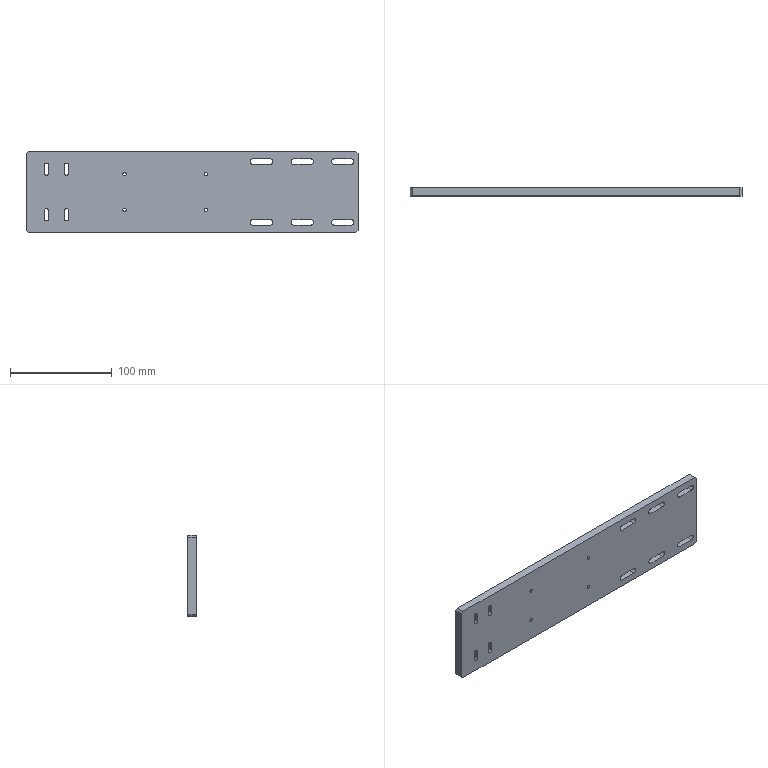Part | STEP file | Y-axis cable chain support plate | 1 solid | 62 faces | box 327 x 8 x 80 mm | volume 201857 mm3 | cylinder 32 | plane 30 | commonest cylinder face diameters 4.5 x12 5.5 x12 3.3 x8